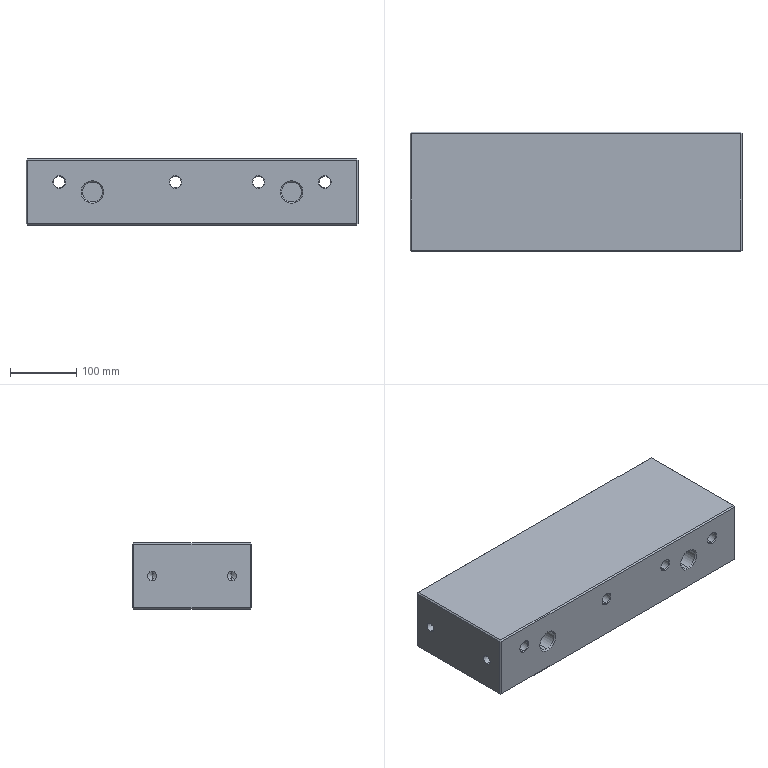Part | STEP file | Spacer block 01 - Tower - 1 cav | 1 solid | 86 faces | box 500 x 180 x 100 mm | volume 8680881 mm3 | cone 32 | plane 30 | cylinder 24 | commonest cylinder face diameters 14 x8 17 x8 30 x8